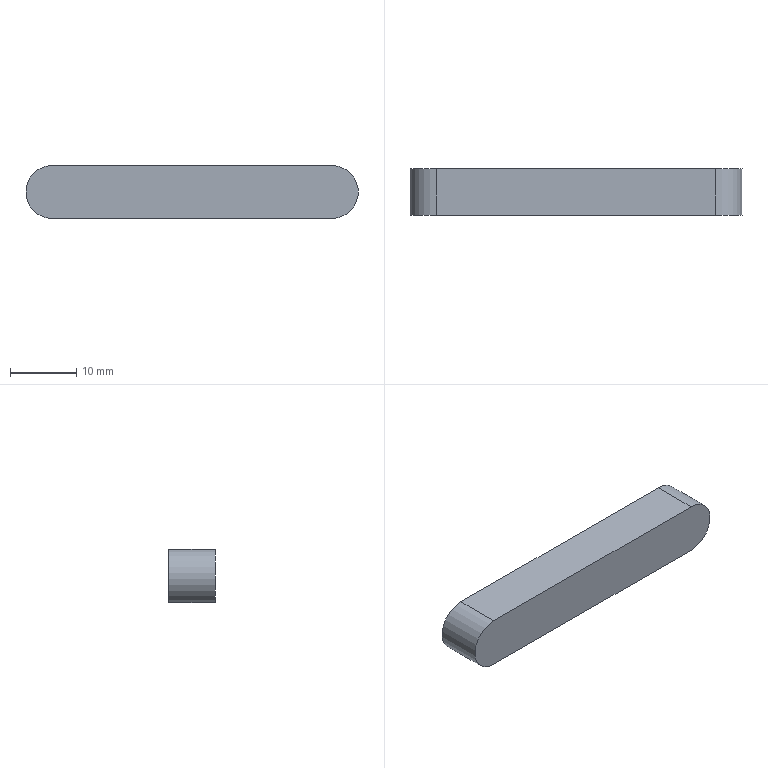Part | SolidWorks | features Extrusion 1, ICE 1 | 1 solid | 632 faces | box 50 x 7 x 8 mm | volume 2702 mm3 | plane 435 | spline 195 | cylinder 2 | commonest cylinder face diameters 8 x2